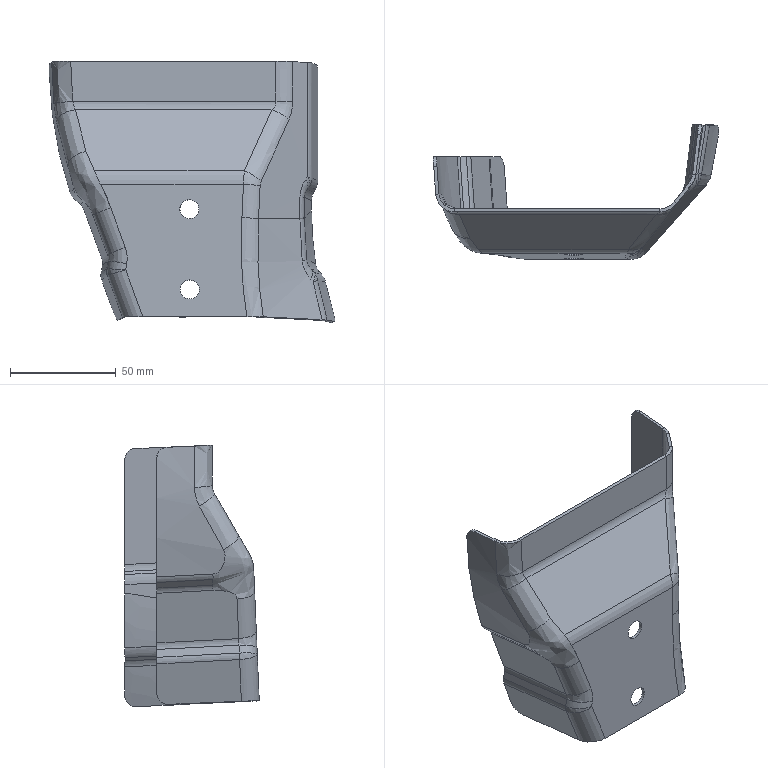Part | STEP file | FNA5401611 | 1 solid | 156 faces | box 135.06 x 63.583 x 123.582 mm | volume 33584 mm3 | spline 128 | cylinder 22 | plane 6 | commonest cylinder face diameters 15 x5 18 x4 16 x3 12 x2 19 x2 9 x1